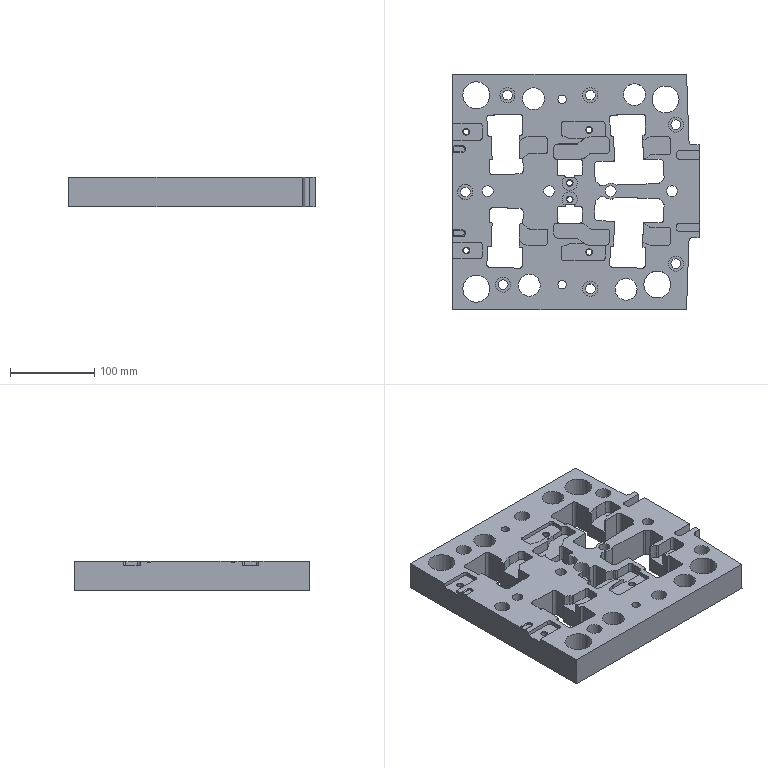Part | NX | features DIE-66 2 | 1 solid | 357 faces | box 293.61 x 280 x 35 mm | volume 1884491 mm3 | plane 171 | cylinder 164 | spline 12 | cone 6 | torus 4 | commonest cylinder face diameters 6 x58 2 x14 18 x13 10 x10 1 x8 4 x8